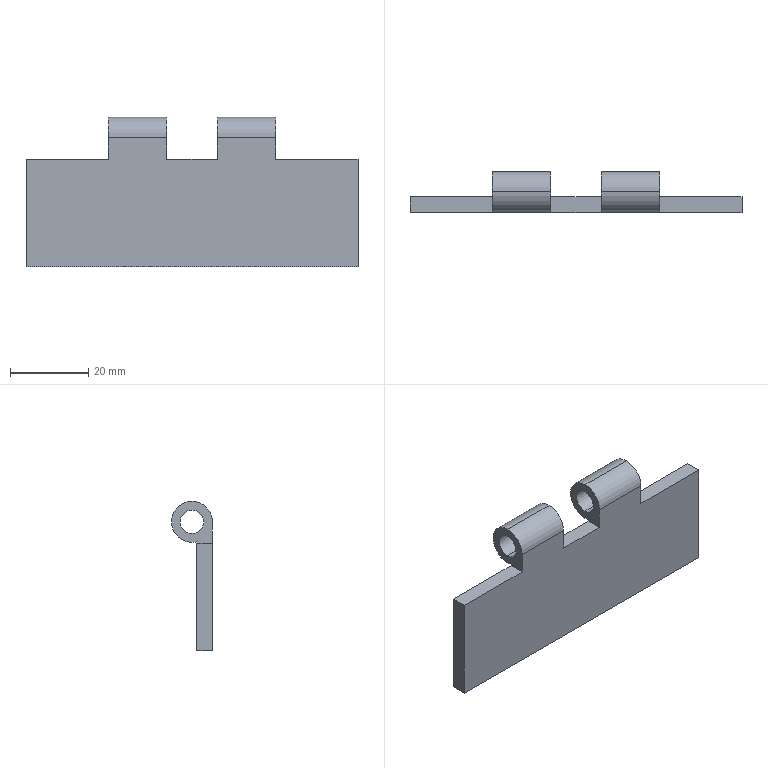Part | SolidWorks | features ICE 2, Chamfer 1, Cut 1, Extrusion 1 | 1 solid | 22 faces | box 85 x 10.5 x 38.25 mm | volume 11305 mm3 | plane 12 | cylinder 10 | commonest cylinder face diameters 10.5 x6 6 x4
STEP:
#1=CARTESIAN_POINT('',(-6.5,0.,-3.));
#2=VERTEX_POINT('',#1);
#3=CARTESIAN_POINT('',(-6.5,0.,3.));
#4=VERTEX_POINT('',#3);
#5=CARTESIAN_POINT('',(-6.5,0.,0.));
#6=DIRECTION('',(-1.,0.,0.));
#7=DIRECTION('',(0.,0.,1.));
#8=AXIS2_PLACEMENT_3D('',#5,#6,#7);
#9=CIRCLE('',#8,3.);
#10=EDGE_CURVE('',#2,#4,#9,.T.);
#11=ORIENTED_EDGE('',*,*,#10,.F.);
#12=CARTESIAN_POINT('',(-21.5,0.,-3.));
#13=VERTEX_POINT('',#12);
#14=CARTESIAN_POINT('',(42.5,0.,-3.));
#15=DIRECTION('',(-1.,0.,0.));
#16=VECTOR('',#15,1000.);
#17=LINE('',#14,#16);
#18=EDGE_CURVE('',#2,#13,#17,.T.);
#19=ORIENTED_EDGE('',*,*,#18,.T.);
#20=CARTESIAN_POINT('',(-21.5,0.,3.));
#21=VERTEX_POINT('',#20);
#22=CARTESIAN_POINT('',(-21.5,0.,0.));
#23=DIRECTION('',(-1.,0.,0.));
#24=DIRECTION('',(0.,0.,1.));
#25=AXIS2_PLACEMENT_3D('',#22,#23,#24);
#26=CIRCLE('',#25,3.);
#27=EDGE_CURVE('',#13,#21,#26,.T.);
#28=ORIENTED_EDGE('',*,*,#27,.T.);
#29=CARTESIAN_POINT('',(42.5,0.,3.));
#30=DIRECTION('',(-1.,0.,0.));
#31=VECTOR('',#30,1000.);
#32=LINE('',#29,#31);
#33=EDGE_CURVE('',#4,#21,#32,.T.);
#34=ORIENTED_EDGE('',*,*,#33,.F.);
#35=EDGE_LOOP('',(#11,#19,#28,#34));
#36=FACE_OUTER_BOUND('',#35,.T.);
#37=CARTESIAN_POINT('',(42.5,0.,0.));
#38=DIRECTION('',(-1.,0.,0.));
#39=DIRECTION('',(0.,0.,1.));
#40=AXIS2_PLACEMENT_3D('',#37,#38,#39);
#41=CYLINDRICAL_SURFACE('',#40,3.);
#42=ADVANCED_FACE('',(#36),#41,.F.);
#43=CARTESIAN_POINT('',(21.5,0.,-3.));
#44=VERTEX_POINT('',#43);
#45=CARTESIAN_POINT('',(21.5,0.,3.));
#46=VERTEX_POINT('',#45);
#47=CARTESIAN_POINT('',(21.5,0.,0.));
#48=DIRECTION('',(-1.,0.,0.));
#49=DIRECTION('',(0.,0.,1.));
#50=AXIS2_PLACEMENT_3D('',#47,#48,#49);
#51=CIRCLE('',#50,3.);
#52=EDGE_CURVE('',#44,#46,#51,.T.);
#53=ORIENTED_EDGE('',*,*,#52,.F.);
#54=CARTESIAN_POINT('',(6.5,0.,-3.));
#55=VERTEX_POINT('',#54);
#56=CARTESIAN_POINT('',(42.5,0.,-3.));
#57=DIRECTION('',(-1.,0.,0.));
#58=VECTOR('',#57,1000.);
#59=LINE('',#56,#58);
#60=EDGE_CURVE('',#44,#55,#59,.T.);
#61=ORIENTED_EDGE('',*,*,#60,.T.);
#62=CARTESIAN_POINT('',(6.5,0.,3.));
#63=VERTEX_POINT('',#62);
#64=CARTESIAN_POINT('',(6.5,0.,0.));
#65=DIRECTION('',(1.,0.,0.));
#66=DIRECTION('',(0.,0.,-1.));
#67=AXIS2_PLACEMENT_3D('',#64,#65,#66);
#68=CIRCLE('',#67,3.);
#69=EDGE_CURVE('',#63,#55,#68,.T.);
#70=ORIENTED_EDGE('',*,*,#69,.F.);
#71=CARTESIAN_POINT('',(42.5,0.,3.));
#72=DIRECTION('',(-1.,0.,0.));
#73=VECTOR('',#72,1000.);
#74=LINE('',#71,#73);
#75=EDGE_CURVE('',#46,#63,#74,.T.);
#76=ORIENTED_EDGE('',*,*,#75,.F.);
#77=EDGE_LOOP('',(#53,#61,#70,#76));
#78=FACE_OUTER_BOUND('',#77,.T.);
#79=CARTESIAN_POINT('',(42.5,0.,0.));
#80=DIRECTION('',(-1.,0.,0.));
#81=DIRECTION('',(0.,0.,1.));
#82=AXIS2_PLACEMENT_3D('',#79,#80,#81);
#83=CYLINDRICAL_SURFACE('',#82,3.);
#84=ADVANCED_FACE('',(#78),#83,.F.);
#85=CARTESIAN_POINT('',(21.5,0.,5.25));
#86=VERTEX_POINT('',#85);
#87=CARTESIAN_POINT('',(21.5,0.,-5.25));
#88=VERTEX_POINT('',#87);
#89=CARTESIAN_POINT('',(21.5,0.,0.));
#90=DIRECTION('',(-1.,0.,0.));
#91=DIRECTION('',(0.,0.,1.));
#92=AXIS2_PLACEMENT_3D('',#89,#90,#91);
#93=CIRCLE('',#92,5.25);
#94=EDGE_CURVE('',#86,#88,#93,.T.);
#95=ORIENTED_EDGE('',*,*,#94,.T.);
#96=CARTESIAN_POINT('',(6.5,0.,-5.25));
#97=VERTEX_POINT('',#96);
#98=CARTESIAN_POINT('',(42.5,0.,-5.25));
#99=DIRECTION('',(-1.,0.,0.));
#100=VECTOR('',#99,1000.);
#101=LINE('',#98,#100);
#102=EDGE_CURVE('',#88,#97,#101,.T.);
#103=ORIENTED_EDGE('',*,*,#102,.T.);
#104=CARTESIAN_POINT('',(6.5,0.,5.25));
#105=VERTEX_POINT('',#104);
#106=CARTESIAN_POINT('',(6.5,0.,0.));
#107=DIRECTION('',(1.,0.,0.));
#108=DIRECTION('',(0.,0.,-1.));
#109=AXIS2_PLACEMENT_3D('',#106,#107,#108);
#110=CIRCLE('',#109,5.25);
#111=EDGE_CURVE('',#97,#105,#110,.T.);
#112=ORIENTED_EDGE('',*,*,#111,.T.);
#113=CARTESIAN_POINT('',(42.5,0.,5.25));
#114=DIRECTION('',(-1.,0.,0.));
#115=VECTOR('',#114,1000.);
#116=LINE('',#113,#115);
#117=EDGE_CURVE('',#86,#105,#116,.T.);
#118=ORIENTED_EDGE('',*,*,#117,.F.);
#119=EDGE_LOOP('',(#95,#103,#112,#118));
#120=FACE_OUTER_BOUND('',#119,.T.);
#121=CARTESIAN_POINT('',(42.5,0.,0.));
#122=DIRECTION('',(-1.,0.,0.));
#123=DIRECTION('',(0.,0.,1.));
#124=AXIS2_PLACEMENT_3D('',#121,#122,#123);
#125=CYLINDRICAL_SURFACE('',#124,5.25);
#126=ADVANCED_FACE('',(#120),#125,.T.);
#127=CARTESIAN_POINT('',(21.5,-5.25,0.));
#128=VERTEX_POINT('',#127);
#129=CARTESIAN_POINT('',(21.5,0.,0.));
#130=DIRECTION('',(-1.,0.,0.));
#131=DIRECTION('',(0.,0.,1.));
#132=AXIS2_PLACEMENT_3D('',#129,#130,#131);
#133=CIRCLE('',#132,5.25);
#134=EDGE_CURVE('',#128,#86,#133,.T.);
#135=ORIENTED_EDGE('',*,*,#134,.T.);
#136=ORIENTED_EDGE('',*,*,#117,.T.);
#137=CARTESIAN_POINT('',(6.5,-5.25,0.));
#138=VERTEX_POINT('',#137);
#139=CARTESIAN_POINT('',(6.5,0.,0.));
#140=DIRECTION('',(1.,0.,0.));
#141=DIRECTION('',(0.,0.,-1.));
#142=AXIS2_PLACEMENT_3D('',#139,#140,#141);
#143=CIRCLE('',#142,5.25);
#144=EDGE_CURVE('',#105,#138,#143,.T.);
#145=ORIENTED_EDGE('',*,*,#144,.T.);
#146=CARTESIAN_POINT('',(42.5,-5.25,0.));
#147=DIRECTION('',(-1.,0.,0.));
#148=VECTOR('',#147,1000.);
#149=LINE('',#146,#148);
#150=EDGE_CURVE('',#128,#138,#149,.T.);
#151=ORIENTED_EDGE('',*,*,#150,.F.);
#152=EDGE_LOOP('',(#135,#136,#145,#151));
#153=FACE_OUTER_BOUND('',#152,.T.);
#154=CARTESIAN_POINT('',(42.5,0.,0.));
#155=DIRECTION('',(-1.,0.,0.));
#156=DIRECTION('',(0.,0.,1.));
#157=AXIS2_PLACEMENT_3D('',#154,#155,#156);
#158=CYLINDRICAL_SURFACE('',#157,5.25);
#159=ADVANCED_FACE('',(#153),#158,.T.);
#160=CARTESIAN_POINT('',(-6.5,0.,5.25));
#161=VERTEX_POINT('',#160);
#162=CARTESIAN_POINT('',(-6.5,0.,-5.25));
#163=VERTEX_POINT('',#162);
#164=CARTESIAN_POINT('',(-6.5,0.,0.));
#165=DIRECTION('',(-1.,0.,0.));
#166=DIRECTION('',(0.,0.,1.));
#167=AXIS2_PLACEMENT_3D('',#164,#165,#166);
#168=CIRCLE('',#167,5.25);
#169=EDGE_CURVE('',#161,#163,#168,.T.);
#170=ORIENTED_EDGE('',*,*,#169,.T.);
#171=CARTESIAN_POINT('',(-21.5,0.,-5.25));
#172=VERTEX_POINT('',#171);
#173=CARTESIAN_POINT('',(42.5,0.,-5.25));
#174=DIRECTION('',(-1.,0.,0.));
#175=VECTOR('',#174,1000.);
#176=LINE('',#173,#175);
#177=EDGE_CURVE('',#163,#172,#176,.T.);
#178=ORIENTED_EDGE('',*,*,#177,.T.);
#179=CARTESIAN_POINT('',(-21.5,0.,5.25));
#180=VERTEX_POINT('',#179);
#181=CARTESIAN_POINT('',(-21.5,0.,0.));
#182=DIRECTION('',(1.,0.,0.));
#183=DIRECTION('',(0.,0.,-1.));
#184=AXIS2_PLACEMENT_3D('',#181,#182,#183);
#185=CIRCLE('',#184,5.25);
#186=EDGE_CURVE('',#172,#180,#185,.T.);
#187=ORIENTED_EDGE('',*,*,#186,.T.);
#188=CARTESIAN_POINT('',(42.5,0.,5.25));
#189=DIRECTION('',(-1.,0.,0.));
#190=VECTOR('',#189,1000.);
#191=LINE('',#188,#190);
#192=EDGE_CURVE('',#161,#180,#191,.T.);
#193=ORIENTED_EDGE('',*,*,#192,.F.);
#194=EDGE_LOOP('',(#170,#178,#187,#193));
#195=FACE_OUTER_BOUND('',#194,.T.);
#196=CARTESIAN_POINT('',(42.5,0.,0.));
#197=DIRECTION('',(-1.,0.,0.));
#198=DIRECTION('',(0.,0.,1.));
#199=AXIS2_PLACEMENT_3D('',#196,#197,#198);
#200=CYLINDRICAL_SURFACE('',#199,5.25);
#201=ADVANCED_FACE('',(#195),#200,.T.);
#202=CARTESIAN_POINT('',(-6.5,-5.25,0.));
#203=VERTEX_POINT('',#202);
#204=CARTESIAN_POINT('',(-6.5,0.,0.));
#205=DIRECTION('',(-1.,0.,0.));
#206=DIRECTION('',(0.,0.,1.));
#207=AXIS2_PLACEMENT_3D('',#204,#205,#206);
#208=CIRCLE('',#207,5.25);
#209=EDGE_CURVE('',#203,#161,#208,.T.);
#210=ORIENTED_EDGE('',*,*,#209,.T.);
#211=ORIENTED_EDGE('',*,*,#192,.T.);
#212=CARTESIAN_POINT('',(-21.5,-5.25,0.));
#213=VERTEX_POINT('',#212);
#214=CARTESIAN_POINT('',(-21.5,0.,0.));
#215=DIRECTION('',(1.,0.,0.));
#216=DIRECTION('',(0.,0.,-1.));
#217=AXIS2_PLACEMENT_3D('',#214,#215,#216);
#218=CIRCLE('',#217,5.25);
#219=EDGE_CURVE('',#180,#213,#218,.T.);
#220=ORIENTED_EDGE('',*,*,#219,.T.);
#221=CARTESIAN_POINT('',(42.5,-5.25,0.));
#222=DIRECTION('',(-1.,0.,0.));
#223=VECTOR('',#222,1000.);
#224=LINE('',#221,#223);
#225=EDGE_CURVE('',#203,#213,#224,.T.);
#226=ORIENTED_EDGE('',*,*,#225,.F.);
#227=EDGE_LOOP('',(#210,#211,#220,#226));
#228=FACE_OUTER_BOUND('',#227,.T.);
#229=CARTESIAN_POINT('',(42.5,0.,0.));
#230=DIRECTION('',(-1.,0.,0.));
#231=DIRECTION('',(0.,0.,1.));
#232=AXIS2_PLACEMENT_3D('',#229,#230,#231);
#233=CYLINDRICAL_SURFACE('',#232,5.25);
#234=ADVANCED_FACE('',(#228),#233,.T.);
#235=ORIENTED_EDGE('',*,*,#177,.F.);
#236=CARTESIAN_POINT('',(-6.5,-1.25,-5.099));
#237=VERTEX_POINT('',#236);
#238=CARTESIAN_POINT('',(-6.5,0.,0.));
#239=DIRECTION('',(-1.,0.,0.));
#240=DIRECTION('',(0.,0.,1.));
#241=AXIS2_PLACEMENT_3D('',#238,#239,#240);
#242=CIRCLE('',#241,5.25);
#243=EDGE_CURVE('',#163,#237,#242,.T.);
#244=ORIENTED_EDGE('',*,*,#243,.T.);
#245=CARTESIAN_POINT('',(-21.5,-1.25,-5.099));
#246=VERTEX_POINT('',#245);
#247=CARTESIAN_POINT('',(42.5,-1.25,-5.099));
#248=DIRECTION('',(-1.,0.,0.));
#249=VECTOR('',#248,1000.);
#250=LINE('',#247,#249);
#251=EDGE_CURVE('',#237,#246,#250,.T.);
#252=ORIENTED_EDGE('',*,*,#251,.T.);
#253=CARTESIAN_POINT('',(-21.5,0.,0.));
#254=DIRECTION('',(1.,0.,0.));
#255=DIRECTION('',(0.,0.,-1.));
#256=AXIS2_PLACEMENT_3D('',#253,#254,#255);
#257=CIRCLE('',#256,5.25);
#258=EDGE_CURVE('',#246,#172,#257,.T.);
#259=ORIENTED_EDGE('',*,*,#258,.T.);
#260=EDGE_LOOP('',(#235,#244,#252,#259));
#261=FACE_OUTER_BOUND('',#260,.T.);
#262=CARTESIAN_POINT('',(42.5,0.,0.));
#263=DIRECTION('',(-1.,0.,0.));
#264=DIRECTION('',(0.,0.,1.));
#265=AXIS2_PLACEMENT_3D('',#262,#263,#264);
#266=CYLINDRICAL_SURFACE('',#265,5.25);
#267=ADVANCED_FACE('',(#261),#266,.T.);
#268=ORIENTED_EDGE('',*,*,#102,.F.);
#269=CARTESIAN_POINT('',(21.5,-1.25,-5.099));
#270=VERTEX_POINT('',#269);
#271=CARTESIAN_POINT('',(21.5,0.,0.));
#272=DIRECTION('',(-1.,0.,0.));
#273=DIRECTION('',(0.,0.,1.));
#274=AXIS2_PLACEMENT_3D('',#271,#272,#273);
#275=CIRCLE('',#274,5.25);
#276=EDGE_CURVE('',#88,#270,#275,.T.);
#277=ORIENTED_EDGE('',*,*,#276,.T.);
#278=CARTESIAN_POINT('',(6.5,-1.25,-5.099));
#279=VERTEX_POINT('',#278);
#280=CARTESIAN_POINT('',(42.5,-1.25,-5.099));
#281=DIRECTION('',(-1.,0.,0.));
#282=VECTOR('',#281,1000.);
#283=LINE('',#280,#282);
#284=EDGE_CURVE('',#270,#279,#283,.T.);
#285=ORIENTED_EDGE('',*,*,#284,.T.);
#286=CARTESIAN_POINT('',(6.5,0.,0.));
#287=DIRECTION('',(1.,0.,0.));
#288=DIRECTION('',(0.,0.,-1.));
#289=AXIS2_PLACEMENT_3D('',#286,#287,#288);
#290=CIRCLE('',#289,5.25);
#291=EDGE_CURVE('',#279,#97,#290,.T.);
#292=ORIENTED_EDGE('',*,*,#291,.T.);
#293=EDGE_LOOP('',(#268,#277,#285,#292));
#294=FACE_OUTER_BOUND('',#293,.T.);
#295=CARTESIAN_POINT('',(42.5,0.,0.));
#296=DIRECTION('',(-1.,0.,0.));
#297=DIRECTION('',(0.,0.,1.));
#298=AXIS2_PLACEMENT_3D('',#295,#296,#297);
#299=CYLINDRICAL_SURFACE('',#298,5.25);
#300=ADVANCED_FACE('',(#294),#299,.T.);
#301=ORIENTED_EDGE('',*,*,#225,.T.);
#302=CARTESIAN_POINT('',(-21.5,-5.25,-5.5));
#303=VERTEX_POINT('',#302);
#304=CARTESIAN_POINT('',(-21.5,-5.25,-33.));
#305=DIRECTION('',(0.,0.,-1.));
#306=VECTOR('',#305,1000.);
#307=LINE('',#304,#306);
#308=EDGE_CURVE('',#213,#303,#307,.T.);
#309=ORIENTED_EDGE('',*,*,#308,.T.);
#310=CARTESIAN_POINT('',(-42.5,-5.25,-5.5));
#311=VERTEX_POINT('',#310);
#312=CARTESIAN_POINT('',(42.5,-5.25,-5.5));
#313=DIRECTION('',(-1.,0.,0.));
#314=VECTOR('',#313,1000.);
#315=LINE('',#312,#314);
#316=EDGE_CURVE('',#303,#311,#315,.T.);
#317=ORIENTED_EDGE('',*,*,#316,.T.);
#318=CARTESIAN_POINT('',(-42.5,-5.25,-33.));
#319=VERTEX_POINT('',#318);
#320=CARTESIAN_POINT('',(-42.5,-5.25,-33.));
#321=DIRECTION('',(0.,0.,-1.));
#322=VECTOR('',#321,1000.);
#323=LINE('',#320,#322);
#324=EDGE_CURVE('',#311,#319,#323,.T.);
#325=ORIENTED_EDGE('',*,*,#324,.T.);
#326=CARTESIAN_POINT('',(42.5,-5.25,-33.));
#327=VERTEX_POINT('',#326);
#328=CARTESIAN_POINT('',(42.5,-5.25,-33.));
#329=DIRECTION('',(-1.,0.,0.));
#330=VECTOR('',#329,1000.);
#331=LINE('',#328,#330);
#332=EDGE_CURVE('',#327,#319,#331,.T.);
#333=ORIENTED_EDGE('',*,*,#332,.F.);
#334=CARTESIAN_POINT('',(42.5,-5.25,-5.5));
#335=VERTEX_POINT('',#334);
#336=CARTESIAN_POINT('',(42.5,-5.25,-33.));
#337=DIRECTION('',(0.,0.,-1.));
#338=VECTOR('',#337,1000.);
#339=LINE('',#336,#338);
#340=EDGE_CURVE('',#335,#327,#339,.T.);
#341=ORIENTED_EDGE('',*,*,#340,.F.);
#342=CARTESIAN_POINT('',(21.5,-5.25,-5.5));
#343=VERTEX_POINT('',#342);
#344=CARTESIAN_POINT('',(42.5,-5.25,-5.5));
#345=DIRECTION('',(-1.,0.,0.));
#346=VECTOR('',#345,1000.);
#347=LINE('',#344,#346);
#348=EDGE_CURVE('',#335,#343,#347,.T.);
#349=ORIENTED_EDGE('',*,*,#348,.T.);
#350=CARTESIAN_POINT('',(21.5,-5.25,-33.));
#351=DIRECTION('',(0.,0.,1.));
#352=VECTOR('',#351,1000.);
#353=LINE('',#350,#352);
#354=EDGE_CURVE('',#343,#128,#353,.T.);
#355=ORIENTED_EDGE('',*,*,#354,.T.);
#356=ORIENTED_EDGE('',*,*,#150,.T.);
#357=CARTESIAN_POINT('',(6.5,-5.25,-5.5));
#358=VERTEX_POINT('',#357);
#359=CARTESIAN_POINT('',(6.5,-5.25,-33.));
#360=DIRECTION('',(0.,0.,-1.));
#361=VECTOR('',#360,1000.);
#362=LINE('',#359,#361);
#363=EDGE_CURVE('',#138,#358,#362,.T.);
#364=ORIENTED_EDGE('',*,*,#363,.T.);
#365=CARTESIAN_POINT('',(-6.5,-5.25,-5.5));
#366=VERTEX_POINT('',#365);
#367=CARTESIAN_POINT('',(42.5,-5.25,-5.5));
#368=DIRECTION('',(-1.,0.,0.));
#369=VECTOR('',#368,1000.);
#370=LINE('',#367,#369);
#371=EDGE_CURVE('',#358,#366,#370,.T.);
#372=ORIENTED_EDGE('',*,*,#371,.T.);
#373=CARTESIAN_POINT('',(-6.5,-5.25,-33.));
#374=DIRECTION('',(0.,0.,1.));
#375=VECTOR('',#374,1000.);
#376=LINE('',#373,#375);
#377=EDGE_CURVE('',#366,#203,#376,.T.);
#378=ORIENTED_EDGE('',*,*,#377,.T.);
#379=EDGE_LOOP('',(#301,#309,#317,#325,#333,#341,#349,#355,#356,#364,#372,#378));
#380=FACE_OUTER_BOUND('',#379,.T.);
#381=CARTESIAN_POINT('',(42.5,-5.25,-33.));
#382=DIRECTION('',(0.,1.,0.));
#383=DIRECTION('',(0.,0.,1.));
#384=AXIS2_PLACEMENT_3D('',#381,#382,#383);
#385=PLANE('',#384);
#386=ADVANCED_FACE('',(#380),#385,.F.);
#387=CARTESIAN_POINT('',(-42.5,-1.25,-33.));
#388=VERTEX_POINT('',#387);
#389=CARTESIAN_POINT('',(-42.5,-5.25,-33.));
#390=DIRECTION('',(0.,1.,0.));
#391=VECTOR('',#390,1000.);
#392=LINE('',#389,#391);
#393=EDGE_CURVE('',#319,#388,#392,.T.);
#394=ORIENTED_EDGE('',*,*,#393,.T.);
#395=CARTESIAN_POINT('',(42.5,-1.25,-33.));
#396=VERTEX_POINT('',#395);
#397=CARTESIAN_POINT('',(42.5,-1.25,-33.));
#398=DIRECTION('',(-1.,0.,0.));
#399=VECTOR('',#398,1000.);
#400=LINE('',#397,#399);
#401=EDGE_CURVE('',#396,#388,#400,.T.);
#402=ORIENTED_EDGE('',*,*,#401,.F.);
#403=CARTESIAN_POINT('',(42.5,-5.25,-33.));
#404=DIRECTION('',(0.,1.,0.));
#405=VECTOR('',#404,1000.);
#406=LINE('',#403,#405);
#407=EDGE_CURVE('',#327,#396,#406,.T.);
#408=ORIENTED_EDGE('',*,*,#407,.F.);
#409=ORIENTED_EDGE('',*,*,#332,.T.);
#410=EDGE_LOOP('',(#394,#402,#408,#409));
#411=FACE_OUTER_BOUND('',#410,.T.);
#412=CARTESIAN_POINT('',(42.5,-5.25,-33.));
#413=DIRECTION('',(0.,0.,1.));
#414=DIRECTION('',(1.,0.,0.));
#415=AXIS2_PLACEMENT_3D('',#412,#413,#414);
#416=PLANE('',#415);
#417=ADVANCED_FACE('',(#411),#416,.F.);
#418=CARTESIAN_POINT('',(-42.5,-1.25,-5.5));
#419=VERTEX_POINT('',#418);
#420=CARTESIAN_POINT('',(-21.5,-1.25,-5.5));
#421=VERTEX_POINT('',#420);
#422=CARTESIAN_POINT('',(42.5,-1.25,-5.5));
#423=DIRECTION('',(1.,0.,0.));
#424=VECTOR('',#423,1000.);
#425=LINE('',#422,#424);
#426=EDGE_CURVE('',#419,#421,#425,.T.);
#427=ORIENTED_EDGE('',*,*,#426,.T.);
#428=CARTESIAN_POINT('',(-21.5,-1.25,-33.));
#429=DIRECTION('',(0.,0.,1.));
#430=VECTOR('',#429,1000.);
#431=LINE('',#428,#430);
#432=EDGE_CURVE('',#421,#246,#431,.T.);
#433=ORIENTED_EDGE('',*,*,#432,.T.);
#434=ORIENTED_EDGE('',*,*,#251,.F.);
#435=CARTESIAN_POINT('',(-6.5,-1.25,-5.5));
#436=VERTEX_POINT('',#435);
#437=CARTESIAN_POINT('',(-6.5,-1.25,-33.));
#438=DIRECTION('',(0.,0.,-1.));
#439=VECTOR('',#438,1000.);
#440=LINE('',#437,#439);
#441=EDGE_CURVE('',#237,#436,#440,.T.);
#442=ORIENTED_EDGE('',*,*,#441,.T.);
#443=CARTESIAN_POINT('',(6.5,-1.25,-5.5));
#444=VERTEX_POINT('',#443);
#445=CARTESIAN_POINT('',(42.5,-1.25,-5.5));
#446=DIRECTION('',(1.,0.,0.));
#447=VECTOR('',#446,1000.);
#448=LINE('',#445,#447);
#449=EDGE_CURVE('',#436,#444,#448,.T.);
#450=ORIENTED_EDGE('',*,*,#449,.T.);
#451=CARTESIAN_POINT('',(6.5,-1.25,-33.));
#452=DIRECTION('',(0.,0.,1.));
#453=VECTOR('',#452,1000.);
#454=LINE('',#451,#453);
#455=EDGE_CURVE('',#444,#279,#454,.T.);
#456=ORIENTED_EDGE('',*,*,#455,.T.);
#457=ORIENTED_EDGE('',*,*,#284,.F.);
#458=CARTESIAN_POINT('',(21.5,-1.25,-5.5));
#459=VERTEX_POINT('',#458);
#460=CARTESIAN_POINT('',(21.5,-1.25,-33.));
#461=DIRECTION('',(0.,0.,-1.));
#462=VECTOR('',#461,1000.);
#463=LINE('',#460,#462);
#464=EDGE_CURVE('',#270,#459,#463,.T.);
#465=ORIENTED_EDGE('',*,*,#464,.T.);
#466=CARTESIAN_POINT('',(42.5,-1.25,-5.5));
#467=VERTEX_POINT('',#466);
#468=CARTESIAN_POINT('',(42.5,-1.25,-5.5));
#469=DIRECTION('',(1.,0.,0.));
#470=VECTOR('',#469,1000.);
#471=LINE('',#468,#470);
#472=EDGE_CURVE('',#459,#467,#471,.T.);
#473=ORIENTED_EDGE('',*,*,#472,.T.);
#474=CARTESIAN_POINT('',(42.5,-1.25,-33.));
#475=DIRECTION('',(0.,0.,1.));
#476=VECTOR('',#475,1000.);
#477=LINE('',#474,#476);
#478=EDGE_CURVE('',#396,#467,#477,.T.);
#479=ORIENTED_EDGE('',*,*,#478,.F.);
#480=ORIENTED_EDGE('',*,*,#401,.T.);
#481=CARTESIAN_POINT('',(-42.5,-1.25,-33.));
#482=DIRECTION('',(0.,0.,1.));
#483=VECTOR('',#482,1000.);
#484=LINE('',#481,#483);
#485=EDGE_CURVE('',#388,#419,#484,.T.);
#486=ORIENTED_EDGE('',*,*,#485,.T.);
#487=EDGE_LOOP('',(#427,#433,#434,#442,#450,#456,#457,#465,#473,#479,#480,#486));
#488=FACE_OUTER_BOUND('',#487,.T.);
#489=CARTESIAN_POINT('',(42.5,-1.25,-33.));
#490=DIRECTION('',(0.,-1.,0.));
#491=DIRECTION('',(0.,0.,-1.));
#492=AXIS2_PLACEMENT_3D('',#489,#490,#491);
#493=PLANE('',#492);
#494=ADVANCED_FACE('',(#488),#493,.F.);
#495=CARTESIAN_POINT('',(42.5,0.,-5.5));
#496=DIRECTION('',(0.,1.,0.));
#497=VECTOR('',#496,1000.);
#498=LINE('',#495,#497);
#499=EDGE_CURVE('',#335,#467,#498,.T.);
#500=ORIENTED_EDGE('',*,*,#499,.F.);
#501=ORIENTED_EDGE('',*,*,#340,.T.);
#502=ORIENTED_EDGE('',*,*,#407,.T.);
#503=ORIENTED_EDGE('',*,*,#478,.T.);
#504=EDGE_LOOP('',(#500,#501,#502,#503));
#505=FACE_OUTER_BOUND('',#504,.T.);
#506=CARTESIAN_POINT('',(42.5,0.,0.));
#507=DIRECTION('',(1.,0.,0.));
#508=DIRECTION('',(0.,0.,-1.));
#509=AXIS2_PLACEMENT_3D('',#506,#507,#508);
#510=PLANE('',#509);
#511=ADVANCED_FACE('',(#505),#510,.T.);
#512=ORIENTED_EDGE('',*,*,#324,.F.);
#513=CARTESIAN_POINT('',(-42.5,0.,-5.5));
#514=DIRECTION('',(0.,1.,0.));
#515=VECTOR('',#514,1000.);
#516=LINE('',#513,#515);
#517=EDGE_CURVE('',#311,#419,#516,.T.);
#518=ORIENTED_EDGE('',*,*,#517,.T.);
#519=ORIENTED_EDGE('',*,*,#485,.F.);
#520=ORIENTED_EDGE('',*,*,#393,.F.);
#521=EDGE_LOOP('',(#512,#518,#519,#520));
#522=FACE_OUTER_BOUND('',#521,.T.);
#523=CARTESIAN_POINT('',(-42.5,0.,0.));
#524=DIRECTION('',(1.,0.,0.));
#525=DIRECTION('',(0.,0.,-1.));
#526=AXIS2_PLACEMENT_3D('',#523,#524,#525);
#527=PLANE('',#526);
#528=ADVANCED_FACE('',(#522),#527,.F.);
#529=CARTESIAN_POINT('',(-21.5,0.,0.));
#530=DIRECTION('',(-1.,0.,0.));
#531=DIRECTION('',(0.,0.,1.));
#532=AXIS2_PLACEMENT_3D('',#529,#530,#531);
#533=CIRCLE('',#532,3.);
#534=EDGE_CURVE('',#21,#13,#533,.T.);
#535=ORIENTED_EDGE('',*,*,#534,.F.);
#536=ORIENTED_EDGE('',*,*,#27,.F.);
#537=EDGE_LOOP('',(#535,#536));
#538=FACE_BOUND('',#537,.T.);
#539=ORIENTED_EDGE('',*,*,#258,.F.);
#540=ORIENTED_EDGE('',*,*,#432,.F.);
#541=CARTESIAN_POINT('',(-21.5,-10.,-5.5));
#542=DIRECTION('',(0.,1.,0.));
#543=VECTOR('',#542,1000.);
#544=LINE('',#541,#543);
#545=EDGE_CURVE('',#303,#421,#544,.T.);
#546=ORIENTED_EDGE('',*,*,#545,.F.);
#547=ORIENTED_EDGE('',*,*,#308,.F.);
#548=ORIENTED_EDGE('',*,*,#219,.F.);
#549=ORIENTED_EDGE('',*,*,#186,.F.);
#550=EDGE_LOOP('',(#539,#540,#546,#547,#548,#549));
#551=FACE_OUTER_BOUND('',#550,.T.);
#552=CARTESIAN_POINT('',(-21.5,-10.,-5.5));
#553=DIRECTION('',(1.,0.,0.));
#554=DIRECTION('',(0.,0.,-1.));
#555=AXIS2_PLACEMENT_3D('',#552,#553,#554);
#556=PLANE('',#555);
#557=ADVANCED_FACE('',(#538,#551),#556,.F.);
#558=ORIENTED_EDGE('',*,*,#545,.T.);
#559=ORIENTED_EDGE('',*,*,#426,.F.);
#560=ORIENTED_EDGE('',*,*,#517,.F.);
#561=ORIENTED_EDGE('',*,*,#316,.F.);
#562=EDGE_LOOP('',(#558,#559,#560,#561));
#563=FACE_OUTER_BOUND('',#562,.T.);
#564=CARTESIAN_POINT('',(-21.5,-10.,-5.5));
#565=DIRECTION('',(0.,0.,-1.));
#566=DIRECTION('',(-1.,0.,0.));
#567=AXIS2_PLACEMENT_3D('',#564,#565,#566);
#568=PLANE('',#567);
#569=ADVANCED_FACE('',(#563),#568,.F.);
#570=CARTESIAN_POINT('',(21.5,0.,0.));
#571=DIRECTION('',(-1.,0.,0.));
#572=DIRECTION('',(0.,0.,1.));
#573=AXIS2_PLACEMENT_3D('',#570,#571,#572);
#574=CIRCLE('',#573,3.);
#575=EDGE_CURVE('',#46,#44,#574,.T.);
#576=ORIENTED_EDGE('',*,*,#575,.T.);
#577=ORIENTED_EDGE('',*,*,#52,.T.);
#578=EDGE_LOOP('',(#576,#577));
#579=FACE_BOUND('',#578,.T.);
#580=CARTESIAN_POINT('',(21.5,-10.,-5.5));
#581=DIRECTION('',(0.,1.,0.));
#582=VECTOR('',#581,1000.);
#583=LINE('',#580,#582);
#584=EDGE_CURVE('',#343,#459,#583,.T.);
#585=ORIENTED_EDGE('',*,*,#584,.T.);
#586=ORIENTED_EDGE('',*,*,#464,.F.);
#587=ORIENTED_EDGE('',*,*,#276,.F.);
#588=ORIENTED_EDGE('',*,*,#94,.F.);
#589=ORIENTED_EDGE('',*,*,#134,.F.);
#590=ORIENTED_EDGE('',*,*,#354,.F.);
#591=EDGE_LOOP('',(#585,#586,#587,#588,#589,#590));
#592=FACE_OUTER_BOUND('',#591,.T.);
#593=CARTESIAN_POINT('',(21.5,-10.,-5.5));
#594=DIRECTION('',(-1.,0.,0.));
#595=DIRECTION('',(0.,0.,1.));
#596=AXIS2_PLACEMENT_3D('',#593,#594,#595);
#597=PLANE('',#596);
#598=ADVANCED_FACE('',(#579,#592),#597,.F.);
#599=ORIENTED_EDGE('',*,*,#499,.T.);
#600=ORIENTED_EDGE('',*,*,#472,.F.);
#601=ORIENTED_EDGE('',*,*,#584,.F.);
#602=ORIENTED_EDGE('',*,*,#348,.F.);
#603=EDGE_LOOP('',(#599,#600,#601,#602));
#604=FACE_OUTER_BOUND('',#603,.T.);
#605=CARTESIAN_POINT('',(21.5,-10.,-5.5));
#606=DIRECTION('',(0.,0.,-1.));
#607=DIRECTION('',(-1.,0.,0.));
#608=AXIS2_PLACEMENT_3D('',#605,#606,#607);
#609=PLANE('',#608);
#610=ADVANCED_FACE('',(#604),#609,.F.);
#611=CARTESIAN_POINT('',(-6.5,0.,0.));
#612=DIRECTION('',(-1.,0.,0.));
#613=DIRECTION('',(0.,0.,1.));
#614=AXIS2_PLACEMENT_3D('',#611,#612,#613);
#615=CIRCLE('',#614,3.);
#616=EDGE_CURVE('',#4,#2,#615,.T.);
#617=ORIENTED_EDGE('',*,*,#616,.T.);
#618=ORIENTED_EDGE('',*,*,#10,.T.);
#619=EDGE_LOOP('',(#617,#618));
#620=FACE_BOUND('',#619,.T.);
#621=CARTESIAN_POINT('',(-6.5,-10.,-5.5));
#622=DIRECTION('',(0.,1.,0.));
#623=VECTOR('',#622,1000.);
#624=LINE('',#621,#623);
#625=EDGE_CURVE('',#366,#436,#624,.T.);
#626=ORIENTED_EDGE('',*,*,#625,.T.);
#627=ORIENTED_EDGE('',*,*,#441,.F.);
#628=ORIENTED_EDGE('',*,*,#243,.F.);
#629=ORIENTED_EDGE('',*,*,#169,.F.);
#630=ORIENTED_EDGE('',*,*,#209,.F.);
#631=ORIENTED_EDGE('',*,*,#377,.F.);
#632=EDGE_LOOP('',(#626,#627,#628,#629,#630,#631));
#633=FACE_OUTER_BOUND('',#632,.T.);
#634=CARTESIAN_POINT('',(-6.5,-10.,-5.5));
#635=DIRECTION('',(-1.,0.,0.));
#636=DIRECTION('',(0.,0.,1.));
#637=AXIS2_PLACEMENT_3D('',#634,#635,#636);
#638=PLANE('',#637);
#639=ADVANCED_FACE('',(#620,#633),#638,.F.);
#640=CARTESIAN_POINT('',(6.5,-10.,-5.5));
#641=DIRECTION('',(0.,1.,0.));
#642=VECTOR('',#641,1000.);
#643=LINE('',#640,#642);
#644=EDGE_CURVE('',#358,#444,#643,.T.);
#645=ORIENTED_EDGE('',*,*,#644,.T.);
#646=ORIENTED_EDGE('',*,*,#449,.F.);
#647=ORIENTED_EDGE('',*,*,#625,.F.);
#648=ORIENTED_EDGE('',*,*,#371,.F.);
#649=EDGE_LOOP('',(#645,#646,#647,#648));
#650=FACE_OUTER_BOUND('',#649,.T.);
#651=CARTESIAN_POINT('',(6.5,-10.,-5.5));
#652=DIRECTION('',(0.,0.,-1.));
#653=DIRECTION('',(-1.,0.,0.));
#654=AXIS2_PLACEMENT_3D('',#651,#652,#653);
#655=PLANE('',#654);
#656=ADVANCED_FACE('',(#650),#655,.F.);
#657=ORIENTED_EDGE('',*,*,#69,.T.);
#658=CARTESIAN_POINT('',(6.5,0.,0.));
#659=DIRECTION('',(1.,0.,0.));
#660=DIRECTION('',(0.,0.,-1.));
#661=AXIS2_PLACEMENT_3D('',#658,#659,#660);
#662=CIRCLE('',#661,3.);
#663=EDGE_CURVE('',#55,#63,#662,.T.);
#664=ORIENTED_EDGE('',*,*,#663,.T.);
#665=EDGE_LOOP('',(#657,#664));
#666=FACE_BOUND('',#665,.T.);
#667=ORIENTED_EDGE('',*,*,#291,.F.);
#668=ORIENTED_EDGE('',*,*,#455,.F.);
#669=ORIENTED_EDGE('',*,*,#644,.F.);
#670=ORIENTED_EDGE('',*,*,#363,.F.);
#671=ORIENTED_EDGE('',*,*,#144,.F.);
#672=ORIENTED_EDGE('',*,*,#111,.F.);
#673=EDGE_LOOP('',(#667,#668,#669,#670,#671,#672));
#674=FACE_OUTER_BOUND('',#673,.T.);
#675=CARTESIAN_POINT('',(6.5,-10.,-5.5));
#676=DIRECTION('',(1.,0.,0.));
#677=DIRECTION('',(0.,0.,-1.));
#678=AXIS2_PLACEMENT_3D('',#675,#676,#677);
#679=PLANE('',#678);
#680=ADVANCED_FACE('',(#666,#674),#679,.F.);
#681=ORIENTED_EDGE('',*,*,#60,.F.);
#682=ORIENTED_EDGE('',*,*,#575,.F.);
#683=ORIENTED_EDGE('',*,*,#75,.T.);
#684=ORIENTED_EDGE('',*,*,#663,.F.);
#685=EDGE_LOOP('',(#681,#682,#683,#684));
#686=FACE_OUTER_BOUND('',#685,.T.);
#687=CARTESIAN_POINT('',(42.5,0.,0.));
#688=DIRECTION('',(-1.,0.,0.));
#689=DIRECTION('',(0.,0.,1.));
#690=AXIS2_PLACEMENT_3D('',#687,#688,#689);
#691=CYLINDRICAL_SURFACE('',#690,3.);
#692=ADVANCED_FACE('',(#686),#691,.F.);
#693=ORIENTED_EDGE('',*,*,#18,.F.);
#694=ORIENTED_EDGE('',*,*,#616,.F.);
#695=ORIENTED_EDGE('',*,*,#33,.T.);
#696=ORIENTED_EDGE('',*,*,#534,.T.);
#697=EDGE_LOOP('',(#693,#694,#695,#696));
#698=FACE_OUTER_BOUND('',#697,.T.);
#699=CARTESIAN_POINT('',(42.5,0.,0.));
#700=DIRECTION('',(-1.,0.,0.));
#701=DIRECTION('',(0.,0.,1.));
#702=AXIS2_PLACEMENT_3D('',#699,#700,#701);
#703=CYLINDRICAL_SURFACE('',#702,3.);
#704=ADVANCED_FACE('',(#698),#703,.F.);
#705=CLOSED_SHELL('',(#42,#84,#126,#159,#201,#234,#267,#300,#386,#417,#494,#511,#528,#557,#569,#598,#610,#639,#656,#680,#692,#704));
#706=MANIFOLD_SOLID_BREP('',#705);
#707=CARTESIAN_POINT('',(0.,0.,0.));
#708=DIRECTION('',(0.,0.,1.));
#709=DIRECTION('',(1.,0.,0.));
#710=AXIS2_PLACEMENT_3D('',#707,#708,#709);
#711=(LENGTH_UNIT()NAMED_UNIT(*)SI_UNIT(.MILLI.,.METRE.));
#712=UNCERTAINTY_MEASURE_WITH_UNIT(LENGTH_MEASURE(0.00001),#711,'','');
#713=(NAMED_UNIT(*)PLANE_ANGLE_UNIT()SI_UNIT($,.RADIAN.));
#714=(NAMED_UNIT(*)SI_UNIT($,.STERADIAN.)SOLID_ANGLE_UNIT());
#715=(GEOMETRIC_REPRESENTATION_CONTEXT(3)GLOBAL_UNCERTAINTY_ASSIGNED_CONTEXT((#712))GLOBAL_UNIT_ASSIGNED_CONTEXT((#711,#713,#714))REPRESENTATION_CONTEXT('',''));
#716=ADVANCED_BREP_SHAPE_REPRESENTATION('',(#706,#710),#715);